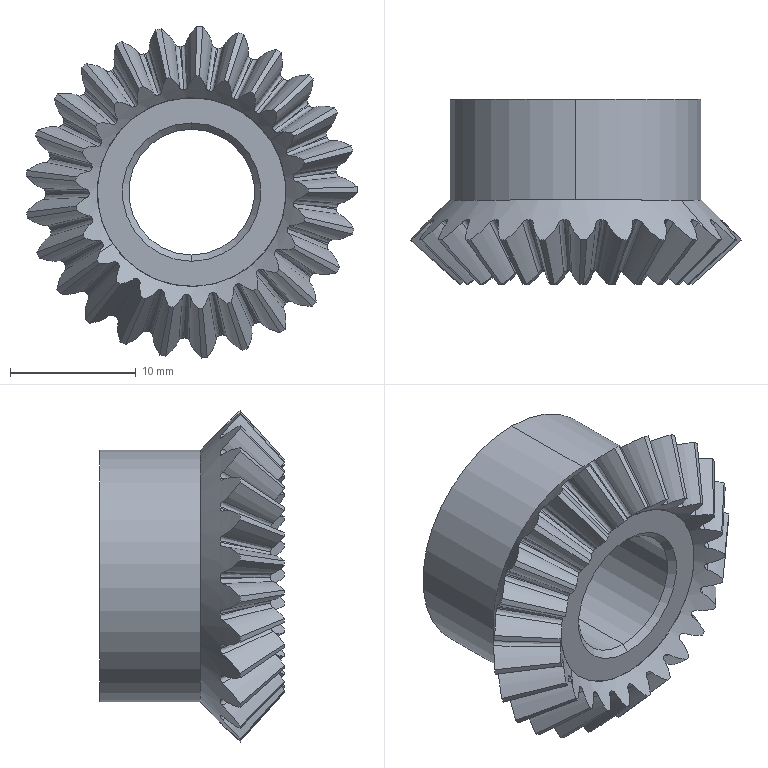Part | SolidWorks | features BaseBody 2 | 2 solids | 170 faces | box 26.356 x 14.7 x 26.386 mm | volume 3537 mm3 | spline 125 | cone 33 | cylinder 8 | plane 4 | commonest cylinder face diameters 15 x4 10 x2 20 x2